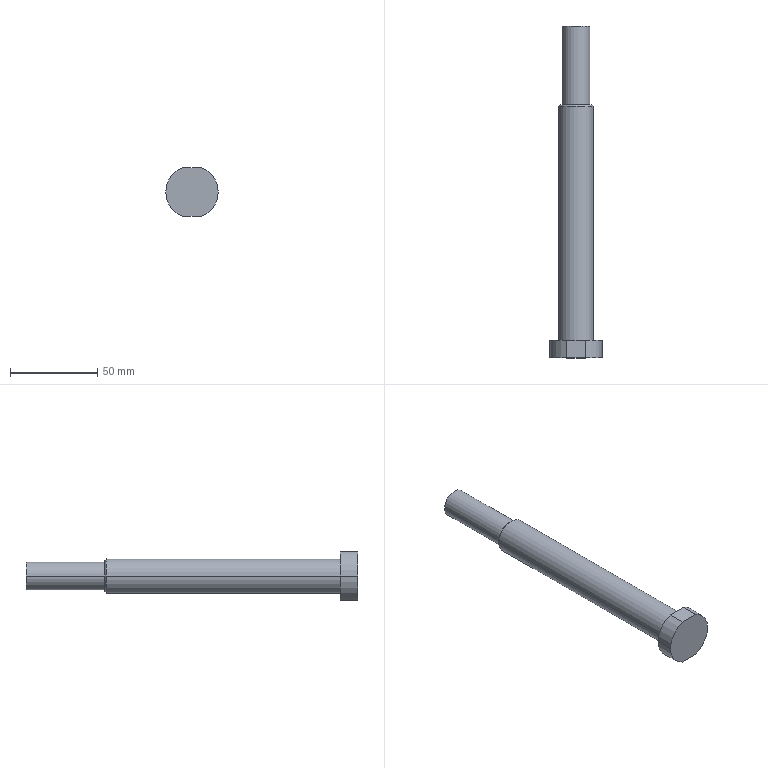Part | SolidWorks | features Chamfer 1, ICE 1, Revolution 1 | 1 solid | 15 faces | box 30 x 190 x 28 mm | volume 58353 mm3 | cylinder 7 | plane 6 | cone 2 | commonest cylinder face diameters 30 x3 16 x2 20 x2
STEP:
#1=CARTESIAN_POINT('',(-9.,50.,0.));
#2=VERTEX_POINT('',#1);
#3=CARTESIAN_POINT('',(9.,50.,0.));
#4=VERTEX_POINT('',#3);
#5=CARTESIAN_POINT('',(0.,50.,0.));
#6=DIRECTION('',(0.,1.,0.));
#7=DIRECTION('',(1.,0.,0.));
#8=AXIS2_PLACEMENT_3D('',#5,#6,#7);
#9=CIRCLE('',#8,9.);
#10=EDGE_CURVE('',#2,#4,#9,.T.);
#11=ORIENTED_EDGE('',*,*,#10,.F.);
#12=CARTESIAN_POINT('',(-10.,49.,0.));
#13=VERTEX_POINT('',#12);
#14=CARTESIAN_POINT('',(-9.,50.,0.));
#15=DIRECTION('',(-0.7071,-0.7071,0.));
#16=VECTOR('',#15,1000.);
#17=LINE('',#14,#16);
#18=EDGE_CURVE('',#2,#13,#17,.T.);
#19=ORIENTED_EDGE('',*,*,#18,.T.);
#20=CARTESIAN_POINT('',(10.,49.,0.));
#21=VERTEX_POINT('',#20);
#22=CARTESIAN_POINT('',(0.,49.,0.));
#23=DIRECTION('',(0.,-1.,0.));
#24=DIRECTION('',(1.,0.,0.));
#25=AXIS2_PLACEMENT_3D('',#22,#23,#24);
#26=CIRCLE('',#25,10.);
#27=EDGE_CURVE('',#21,#13,#26,.T.);
#28=ORIENTED_EDGE('',*,*,#27,.F.);
#29=CARTESIAN_POINT('',(9.,50.,0.));
#30=DIRECTION('',(0.7071,-0.7071,0.));
#31=VECTOR('',#30,1000.);
#32=LINE('',#29,#31);
#33=EDGE_CURVE('',#4,#21,#32,.T.);
#34=ORIENTED_EDGE('',*,*,#33,.F.);
#35=EDGE_LOOP('',(#11,#19,#28,#34));
#36=FACE_OUTER_BOUND('',#35,.T.);
#37=CARTESIAN_POINT('',(0.,50.,0.));
#38=DIRECTION('',(0.,-1.,0.));
#39=DIRECTION('',(1.,0.,0.));
#40=AXIS2_PLACEMENT_3D('',#37,#38,#39);
#41=CONICAL_SURFACE('',#40,9.,0.7854);
#42=ADVANCED_FACE('',(#36),#41,.T.);
#43=CARTESIAN_POINT('',(-8.,50.,0.));
#44=VERTEX_POINT('',#43);
#45=CARTESIAN_POINT('',(8.,50.,0.));
#46=VERTEX_POINT('',#45);
#47=CARTESIAN_POINT('',(0.,50.,0.));
#48=DIRECTION('',(0.,1.,0.));
#49=DIRECTION('',(-1.,0.,0.));
#50=AXIS2_PLACEMENT_3D('',#47,#48,#49);
#51=CIRCLE('',#50,8.);
#52=EDGE_CURVE('',#44,#46,#51,.T.);
#53=ORIENTED_EDGE('',*,*,#52,.T.);
#54=CARTESIAN_POINT('',(8.,95.,0.));
#55=VERTEX_POINT('',#54);
#56=CARTESIAN_POINT('',(8.,95.,0.));
#57=DIRECTION('',(0.,1.,0.));
#58=VECTOR('',#57,1000.);
#59=LINE('',#56,#58);
#60=EDGE_CURVE('',#46,#55,#59,.T.);
#61=ORIENTED_EDGE('',*,*,#60,.T.);
#62=CARTESIAN_POINT('',(-8.,95.,0.));
#63=VERTEX_POINT('',#62);
#64=CARTESIAN_POINT('',(0.,95.,0.));
#65=DIRECTION('',(0.,1.,0.));
#66=DIRECTION('',(-1.,0.,0.));
#67=AXIS2_PLACEMENT_3D('',#64,#65,#66);
#68=CIRCLE('',#67,8.);
#69=EDGE_CURVE('',#63,#55,#68,.T.);
#70=ORIENTED_EDGE('',*,*,#69,.F.);
#71=CARTESIAN_POINT('',(-8.,95.,0.));
#72=DIRECTION('',(0.,1.,0.));
#73=VECTOR('',#72,1000.);
#74=LINE('',#71,#73);
#75=EDGE_CURVE('',#44,#63,#74,.T.);
#76=ORIENTED_EDGE('',*,*,#75,.F.);
#77=EDGE_LOOP('',(#53,#61,#70,#76));
#78=FACE_OUTER_BOUND('',#77,.T.);
#79=CARTESIAN_POINT('',(0.,95.,0.));
#80=DIRECTION('',(0.,1.,0.));
#81=DIRECTION('',(-1.,0.,0.));
#82=AXIS2_PLACEMENT_3D('',#79,#80,#81);
#83=CYLINDRICAL_SURFACE('',#82,8.);
#84=ADVANCED_FACE('',(#78),#83,.T.);
#85=CARTESIAN_POINT('',(-10.,-85.,0.));
#86=VERTEX_POINT('',#85);
#87=CARTESIAN_POINT('',(10.,-85.,0.));
#88=VERTEX_POINT('',#87);
#89=CARTESIAN_POINT('',(0.,-85.,0.));
#90=DIRECTION('',(0.,1.,0.));
#91=DIRECTION('',(-1.,0.,0.));
#92=AXIS2_PLACEMENT_3D('',#89,#90,#91);
#93=CIRCLE('',#92,10.);
#94=EDGE_CURVE('',#86,#88,#93,.T.);
#95=ORIENTED_EDGE('',*,*,#94,.T.);
#96=CARTESIAN_POINT('',(10.,95.,0.));
#97=DIRECTION('',(0.,1.,0.));
#98=VECTOR('',#97,1000.);
#99=LINE('',#96,#98);
#100=EDGE_CURVE('',#88,#21,#99,.T.);
#101=ORIENTED_EDGE('',*,*,#100,.T.);
#102=ORIENTED_EDGE('',*,*,#27,.T.);
#103=CARTESIAN_POINT('',(-10.,95.,0.));
#104=DIRECTION('',(0.,1.,0.));
#105=VECTOR('',#104,1000.);
#106=LINE('',#103,#105);
#107=EDGE_CURVE('',#86,#13,#106,.T.);
#108=ORIENTED_EDGE('',*,*,#107,.F.);
#109=EDGE_LOOP('',(#95,#101,#102,#108));
#110=FACE_OUTER_BOUND('',#109,.T.);
#111=CARTESIAN_POINT('',(0.,95.,0.));
#112=DIRECTION('',(0.,1.,0.));
#113=DIRECTION('',(-1.,0.,0.));
#114=AXIS2_PLACEMENT_3D('',#111,#112,#113);
#115=CYLINDRICAL_SURFACE('',#114,10.);
#116=ADVANCED_FACE('',(#110),#115,.T.);
#117=CARTESIAN_POINT('',(-5.385,-95.,-14.));
#118=VERTEX_POINT('',#117);
#119=CARTESIAN_POINT('',(-15.,-95.,0.));
#120=VERTEX_POINT('',#119);
#121=CARTESIAN_POINT('',(0.,-95.,0.));
#122=DIRECTION('',(0.,1.,0.));
#123=DIRECTION('',(-1.,0.,0.));
#124=AXIS2_PLACEMENT_3D('',#121,#122,#123);
#125=CIRCLE('',#124,15.);
#126=EDGE_CURVE('',#118,#120,#125,.T.);
#127=ORIENTED_EDGE('',*,*,#126,.T.);
#128=CARTESIAN_POINT('',(-15.,-85.,0.));
#129=VERTEX_POINT('',#128);
#130=CARTESIAN_POINT('',(-15.,95.,0.));
#131=DIRECTION('',(0.,1.,0.));
#132=VECTOR('',#131,1000.);
#133=LINE('',#130,#132);
#134=EDGE_CURVE('',#120,#129,#133,.T.);
#135=ORIENTED_EDGE('',*,*,#134,.T.);
#136=CARTESIAN_POINT('',(-5.385,-85.,-14.));
#137=VERTEX_POINT('',#136);
#138=CARTESIAN_POINT('',(0.,-85.,0.));
#139=DIRECTION('',(0.,1.,0.));
#140=DIRECTION('',(-1.,0.,0.));
#141=AXIS2_PLACEMENT_3D('',#138,#139,#140);
#142=CIRCLE('',#141,15.);
#143=EDGE_CURVE('',#137,#129,#142,.T.);
#144=ORIENTED_EDGE('',*,*,#143,.F.);
#145=CARTESIAN_POINT('',(-5.385,95.,-14.));
#146=DIRECTION('',(0.,-1.,0.));
#147=VECTOR('',#146,1000.);
#148=LINE('',#145,#147);
#149=EDGE_CURVE('',#137,#118,#148,.T.);
#150=ORIENTED_EDGE('',*,*,#149,.T.);
#151=EDGE_LOOP('',(#127,#135,#144,#150));
#152=FACE_OUTER_BOUND('',#151,.T.);
#153=CARTESIAN_POINT('',(0.,95.,0.));
#154=DIRECTION('',(0.,1.,0.));
#155=DIRECTION('',(-1.,0.,0.));
#156=AXIS2_PLACEMENT_3D('',#153,#154,#155);
#157=CYLINDRICAL_SURFACE('',#156,15.);
#158=ADVANCED_FACE('',(#152),#157,.T.);
#159=ORIENTED_EDGE('',*,*,#134,.F.);
#160=CARTESIAN_POINT('',(-5.385,-95.,14.));
#161=VERTEX_POINT('',#160);
#162=CARTESIAN_POINT('',(0.,-95.,0.));
#163=DIRECTION('',(0.,1.,0.));
#164=DIRECTION('',(-1.,0.,0.));
#165=AXIS2_PLACEMENT_3D('',#162,#163,#164);
#166=CIRCLE('',#165,15.);
#167=EDGE_CURVE('',#120,#161,#166,.T.);
#168=ORIENTED_EDGE('',*,*,#167,.T.);
#169=CARTESIAN_POINT('',(-5.385,-85.,14.));
#170=VERTEX_POINT('',#169);
#171=CARTESIAN_POINT('',(-5.385,95.,14.));
#172=DIRECTION('',(0.,1.,0.));
#173=VECTOR('',#172,1000.);
#174=LINE('',#171,#173);
#175=EDGE_CURVE('',#161,#170,#174,.T.);
#176=ORIENTED_EDGE('',*,*,#175,.T.);
#177=CARTESIAN_POINT('',(0.,-85.,0.));
#178=DIRECTION('',(0.,1.,0.));
#179=DIRECTION('',(-1.,0.,0.));
#180=AXIS2_PLACEMENT_3D('',#177,#178,#179);
#181=CIRCLE('',#180,15.);
#182=EDGE_CURVE('',#129,#170,#181,.T.);
#183=ORIENTED_EDGE('',*,*,#182,.F.);
#184=EDGE_LOOP('',(#159,#168,#176,#183));
#185=FACE_OUTER_BOUND('',#184,.T.);
#186=CARTESIAN_POINT('',(0.,95.,0.));
#187=DIRECTION('',(0.,1.,0.));
#188=DIRECTION('',(-1.,0.,0.));
#189=AXIS2_PLACEMENT_3D('',#186,#187,#188);
#190=CYLINDRICAL_SURFACE('',#189,15.);
#191=ADVANCED_FACE('',(#185),#190,.T.);
#192=CARTESIAN_POINT('',(5.385,-85.,14.));
#193=VERTEX_POINT('',#192);
#194=CARTESIAN_POINT('',(5.385,-85.,-14.));
#195=VERTEX_POINT('',#194);
#196=CARTESIAN_POINT('',(0.,-85.,0.));
#197=DIRECTION('',(0.,1.,0.));
#198=DIRECTION('',(-1.,0.,0.));
#199=AXIS2_PLACEMENT_3D('',#196,#197,#198);
#200=CIRCLE('',#199,15.);
#201=EDGE_CURVE('',#193,#195,#200,.T.);
#202=ORIENTED_EDGE('',*,*,#201,.F.);
#203=CARTESIAN_POINT('',(5.385,-95.,14.));
#204=VERTEX_POINT('',#203);
#205=CARTESIAN_POINT('',(5.385,95.,14.));
#206=DIRECTION('',(0.,-1.,0.));
#207=VECTOR('',#206,1000.);
#208=LINE('',#205,#207);
#209=EDGE_CURVE('',#193,#204,#208,.T.);
#210=ORIENTED_EDGE('',*,*,#209,.T.);
#211=CARTESIAN_POINT('',(5.385,-95.,-14.));
#212=VERTEX_POINT('',#211);
#213=CARTESIAN_POINT('',(0.,-95.,0.));
#214=DIRECTION('',(0.,1.,0.));
#215=DIRECTION('',(-1.,0.,0.));
#216=AXIS2_PLACEMENT_3D('',#213,#214,#215);
#217=CIRCLE('',#216,15.);
#218=EDGE_CURVE('',#204,#212,#217,.T.);
#219=ORIENTED_EDGE('',*,*,#218,.T.);
#220=CARTESIAN_POINT('',(5.385,95.,-14.));
#221=DIRECTION('',(0.,1.,0.));
#222=VECTOR('',#221,1000.);
#223=LINE('',#220,#222);
#224=EDGE_CURVE('',#212,#195,#223,.T.);
#225=ORIENTED_EDGE('',*,*,#224,.T.);
#226=EDGE_LOOP('',(#202,#210,#219,#225));
#227=FACE_OUTER_BOUND('',#226,.T.);
#228=CARTESIAN_POINT('',(0.,95.,0.));
#229=DIRECTION('',(0.,1.,0.));
#230=DIRECTION('',(-1.,0.,0.));
#231=AXIS2_PLACEMENT_3D('',#228,#229,#230);
#232=CYLINDRICAL_SURFACE('',#231,15.);
#233=ADVANCED_FACE('',(#227),#232,.T.);
#234=ORIENTED_EDGE('',*,*,#94,.F.);
#235=CARTESIAN_POINT('',(0.,-85.,0.));
#236=DIRECTION('',(0.,1.,0.));
#237=DIRECTION('',(-1.,0.,0.));
#238=AXIS2_PLACEMENT_3D('',#235,#236,#237);
#239=CIRCLE('',#238,10.);
#240=EDGE_CURVE('',#88,#86,#239,.T.);
#241=ORIENTED_EDGE('',*,*,#240,.F.);
#242=EDGE_LOOP('',(#234,#241));
#243=FACE_BOUND('',#242,.T.);
#244=ORIENTED_EDGE('',*,*,#143,.T.);
#245=ORIENTED_EDGE('',*,*,#182,.T.);
#246=CARTESIAN_POINT('',(16.919,-85.,14.));
#247=DIRECTION('',(-1.,0.,0.));
#248=VECTOR('',#247,1000.);
#249=LINE('',#246,#248);
#250=EDGE_CURVE('',#193,#170,#249,.T.);
#251=ORIENTED_EDGE('',*,*,#250,.F.);
#252=ORIENTED_EDGE('',*,*,#201,.T.);
#253=CARTESIAN_POINT('',(20.445,-85.,-14.));
#254=DIRECTION('',(1.,0.,0.));
#255=VECTOR('',#254,1000.);
#256=LINE('',#253,#255);
#257=EDGE_CURVE('',#137,#195,#256,.T.);
#258=ORIENTED_EDGE('',*,*,#257,.F.);
#259=EDGE_LOOP('',(#244,#245,#251,#252,#258));
#260=FACE_OUTER_BOUND('',#259,.T.);
#261=CARTESIAN_POINT('',(15.,-85.,0.));
#262=DIRECTION('',(0.,-1.,0.));
#263=DIRECTION('',(1.,0.,0.));
#264=AXIS2_PLACEMENT_3D('',#261,#262,#263);
#265=PLANE('',#264);
#266=ADVANCED_FACE('',(#243,#260),#265,.F.);
#267=ORIENTED_EDGE('',*,*,#100,.F.);
#268=ORIENTED_EDGE('',*,*,#240,.T.);
#269=ORIENTED_EDGE('',*,*,#107,.T.);
#270=CARTESIAN_POINT('',(0.,49.,0.));
#271=DIRECTION('',(0.,-1.,0.));
#272=DIRECTION('',(1.,0.,0.));
#273=AXIS2_PLACEMENT_3D('',#270,#271,#272);
#274=CIRCLE('',#273,10.);
#275=EDGE_CURVE('',#13,#21,#274,.T.);
#276=ORIENTED_EDGE('',*,*,#275,.T.);
#277=EDGE_LOOP('',(#267,#268,#269,#276));
#278=FACE_OUTER_BOUND('',#277,.T.);
#279=CARTESIAN_POINT('',(0.,95.,0.));
#280=DIRECTION('',(0.,1.,0.));
#281=DIRECTION('',(-1.,0.,0.));
#282=AXIS2_PLACEMENT_3D('',#279,#280,#281);
#283=CYLINDRICAL_SURFACE('',#282,10.);
#284=ADVANCED_FACE('',(#278),#283,.T.);
#285=CARTESIAN_POINT('',(0.,50.,0.));
#286=DIRECTION('',(0.,1.,0.));
#287=DIRECTION('',(1.,0.,0.));
#288=AXIS2_PLACEMENT_3D('',#285,#286,#287);
#289=CIRCLE('',#288,9.);
#290=EDGE_CURVE('',#4,#2,#289,.T.);
#291=ORIENTED_EDGE('',*,*,#290,.T.);
#292=ORIENTED_EDGE('',*,*,#10,.T.);
#293=EDGE_LOOP('',(#291,#292));
#294=FACE_OUTER_BOUND('',#293,.T.);
#295=ORIENTED_EDGE('',*,*,#52,.F.);
#296=CARTESIAN_POINT('',(0.,50.,0.));
#297=DIRECTION('',(0.,1.,0.));
#298=DIRECTION('',(-1.,0.,0.));
#299=AXIS2_PLACEMENT_3D('',#296,#297,#298);
#300=CIRCLE('',#299,8.);
#301=EDGE_CURVE('',#46,#44,#300,.T.);
#302=ORIENTED_EDGE('',*,*,#301,.F.);
#303=EDGE_LOOP('',(#295,#302));
#304=FACE_BOUND('',#303,.T.);
#305=CARTESIAN_POINT('',(10.,50.,0.));
#306=DIRECTION('',(0.,-1.,0.));
#307=DIRECTION('',(1.,0.,0.));
#308=AXIS2_PLACEMENT_3D('',#305,#306,#307);
#309=PLANE('',#308);
#310=ADVANCED_FACE('',(#294,#304),#309,.F.);
#311=ORIENTED_EDGE('',*,*,#60,.F.);
#312=ORIENTED_EDGE('',*,*,#301,.T.);
#313=ORIENTED_EDGE('',*,*,#75,.T.);
#314=CARTESIAN_POINT('',(0.,95.,0.));
#315=DIRECTION('',(0.,1.,0.));
#316=DIRECTION('',(-1.,0.,0.));
#317=AXIS2_PLACEMENT_3D('',#314,#315,#316);
#318=CIRCLE('',#317,8.);
#319=EDGE_CURVE('',#55,#63,#318,.T.);
#320=ORIENTED_EDGE('',*,*,#319,.F.);
#321=EDGE_LOOP('',(#311,#312,#313,#320));
#322=FACE_OUTER_BOUND('',#321,.T.);
#323=CARTESIAN_POINT('',(0.,95.,0.));
#324=DIRECTION('',(0.,1.,0.));
#325=DIRECTION('',(-1.,0.,0.));
#326=AXIS2_PLACEMENT_3D('',#323,#324,#325);
#327=CYLINDRICAL_SURFACE('',#326,8.);
#328=ADVANCED_FACE('',(#322),#327,.T.);
#329=ORIENTED_EDGE('',*,*,#69,.T.);
#330=ORIENTED_EDGE('',*,*,#319,.T.);
#331=EDGE_LOOP('',(#329,#330));
#332=FACE_OUTER_BOUND('',#331,.T.);
#333=CARTESIAN_POINT('',(8.,95.,0.));
#334=DIRECTION('',(0.,-1.,0.));
#335=DIRECTION('',(1.,0.,0.));
#336=AXIS2_PLACEMENT_3D('',#333,#334,#335);
#337=PLANE('',#336);
#338=ADVANCED_FACE('',(#332),#337,.F.);
#339=ORIENTED_EDGE('',*,*,#218,.F.);
#340=CARTESIAN_POINT('',(0.,-95.,14.));
#341=DIRECTION('',(-1.,0.,0.));
#342=VECTOR('',#341,1000.);
#343=LINE('',#340,#342);
#344=EDGE_CURVE('',#204,#161,#343,.T.);
#345=ORIENTED_EDGE('',*,*,#344,.T.);
#346=ORIENTED_EDGE('',*,*,#167,.F.);
#347=ORIENTED_EDGE('',*,*,#126,.F.);
#348=CARTESIAN_POINT('',(0.,-95.,-14.));
#349=DIRECTION('',(1.,0.,0.));
#350=VECTOR('',#349,1000.);
#351=LINE('',#348,#350);
#352=EDGE_CURVE('',#118,#212,#351,.T.);
#353=ORIENTED_EDGE('',*,*,#352,.T.);
#354=EDGE_LOOP('',(#339,#345,#346,#347,#353));
#355=FACE_OUTER_BOUND('',#354,.T.);
#356=CARTESIAN_POINT('',(0.,-95.,0.));
#357=DIRECTION('',(0.,1.,0.));
#358=DIRECTION('',(-1.,0.,0.));
#359=AXIS2_PLACEMENT_3D('',#356,#357,#358);
#360=PLANE('',#359);
#361=ADVANCED_FACE('',(#355),#360,.F.);
#362=ORIENTED_EDGE('',*,*,#18,.F.);
#363=ORIENTED_EDGE('',*,*,#290,.F.);
#364=ORIENTED_EDGE('',*,*,#33,.T.);
#365=ORIENTED_EDGE('',*,*,#275,.F.);
#366=EDGE_LOOP('',(#362,#363,#364,#365));
#367=FACE_OUTER_BOUND('',#366,.T.);
#368=CARTESIAN_POINT('',(0.,50.,0.));
#369=DIRECTION('',(0.,-1.,0.));
#370=DIRECTION('',(1.,0.,0.));
#371=AXIS2_PLACEMENT_3D('',#368,#369,#370);
#372=CONICAL_SURFACE('',#371,9.,0.7854);
#373=ADVANCED_FACE('',(#367),#372,.T.);
#374=ORIENTED_EDGE('',*,*,#352,.F.);
#375=ORIENTED_EDGE('',*,*,#149,.F.);
#376=ORIENTED_EDGE('',*,*,#257,.T.);
#377=ORIENTED_EDGE('',*,*,#224,.F.);
#378=EDGE_LOOP('',(#374,#375,#376,#377));
#379=FACE_OUTER_BOUND('',#378,.T.);
#380=CARTESIAN_POINT('',(20.445,-115.,-14.));
#381=DIRECTION('',(0.,0.,1.));
#382=DIRECTION('',(1.,0.,0.));
#383=AXIS2_PLACEMENT_3D('',#380,#381,#382);
#384=PLANE('',#383);
#385=ADVANCED_FACE('',(#379),#384,.F.);
#386=ORIENTED_EDGE('',*,*,#344,.F.);
#387=ORIENTED_EDGE('',*,*,#209,.F.);
#388=ORIENTED_EDGE('',*,*,#250,.T.);
#389=ORIENTED_EDGE('',*,*,#175,.F.);
#390=EDGE_LOOP('',(#386,#387,#388,#389));
#391=FACE_OUTER_BOUND('',#390,.T.);
#392=CARTESIAN_POINT('',(16.919,-115.,14.));
#393=DIRECTION('',(0.,0.,-1.));
#394=DIRECTION('',(-1.,0.,0.));
#395=AXIS2_PLACEMENT_3D('',#392,#393,#394);
#396=PLANE('',#395);
#397=ADVANCED_FACE('',(#391),#396,.F.);
#398=CLOSED_SHELL('',(#42,#84,#116,#158,#191,#233,#266,#284,#310,#328,#338,#361,#373,#385,#397));
#399=MANIFOLD_SOLID_BREP('',#398);
#400=CARTESIAN_POINT('',(0.,0.,0.));
#401=DIRECTION('',(0.,0.,1.));
#402=DIRECTION('',(1.,0.,0.));
#403=AXIS2_PLACEMENT_3D('',#400,#401,#402);
#404=(LENGTH_UNIT()NAMED_UNIT(*)SI_UNIT(.MILLI.,.METRE.));
#405=UNCERTAINTY_MEASURE_WITH_UNIT(LENGTH_MEASURE(0.00001),#404,'','');
#406=(NAMED_UNIT(*)PLANE_ANGLE_UNIT()SI_UNIT($,.RADIAN.));
#407=(NAMED_UNIT(*)SI_UNIT($,.STERADIAN.)SOLID_ANGLE_UNIT());
#408=(GEOMETRIC_REPRESENTATION_CONTEXT(3)GLOBAL_UNCERTAINTY_ASSIGNED_CONTEXT((#405))GLOBAL_UNIT_ASSIGNED_CONTEXT((#404,#406,#407))REPRESENTATION_CONTEXT('',''));
#409=ADVANCED_BREP_SHAPE_REPRESENTATION('',(#399,#403),#408);